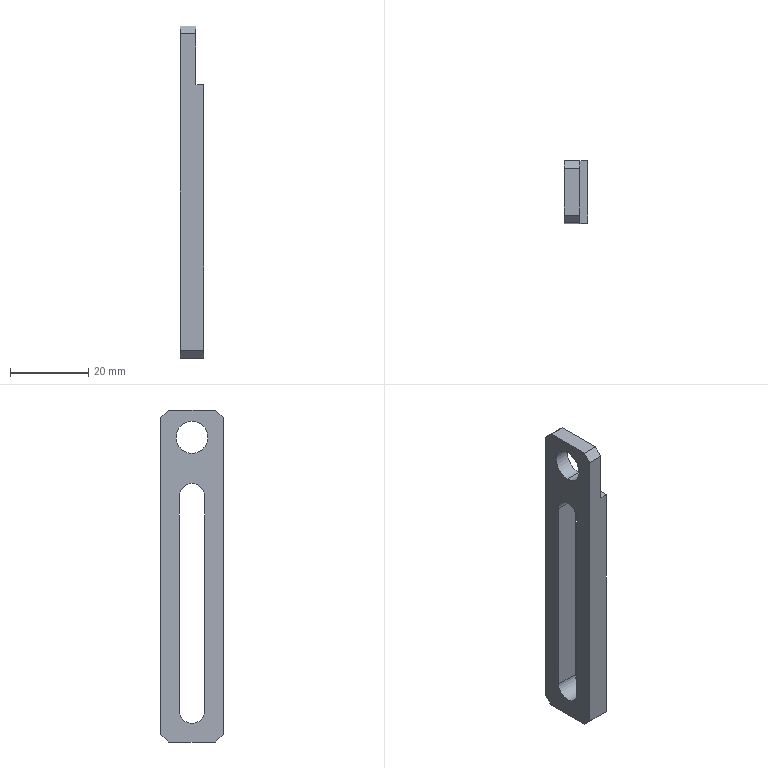Part | SolidWorks | features Chamfer 1, Extrusion 1, HoleWzd 1, ICE 1 | 1 solid | 19 faces | box 6 x 16 x 85 mm | volume 5085 mm3 | plane 14 | cylinder 5 | commonest cylinder face diameters 6.5 x3 8.2 x2
STEP:
#1=CARTESIAN_POINT('',(0.,-8.,-2.9));
#2=VERTEX_POINT('',#1);
#3=CARTESIAN_POINT('',(0.,-8.,-11.1));
#4=VERTEX_POINT('',#3);
#5=CARTESIAN_POINT('',(0.,-8.,-7.));
#6=DIRECTION('',(1.,0.,0.));
#7=DIRECTION('',(0.,0.,-1.));
#8=AXIS2_PLACEMENT_3D('',#5,#6,#7);
#9=CIRCLE('',#8,4.1);
#10=EDGE_CURVE('',#2,#4,#9,.T.);
#11=ORIENTED_EDGE('',*,*,#10,.F.);
#12=CARTESIAN_POINT('',(4.,-8.,-2.9));
#13=VERTEX_POINT('',#12);
#14=CARTESIAN_POINT('',(6.,-8.,-2.9));
#15=DIRECTION('',(1.,0.,0.));
#16=VECTOR('',#15,1000.);
#17=LINE('',#14,#16);
#18=EDGE_CURVE('',#2,#13,#17,.T.);
#19=ORIENTED_EDGE('',*,*,#18,.T.);
#20=CARTESIAN_POINT('',(4.,-8.,-11.1));
#21=VERTEX_POINT('',#20);
#22=CARTESIAN_POINT('',(4.,-8.,-7.));
#23=DIRECTION('',(1.,0.,0.));
#24=DIRECTION('',(0.,0.,1.));
#25=AXIS2_PLACEMENT_3D('',#22,#23,#24);
#26=CIRCLE('',#25,4.1);
#27=EDGE_CURVE('',#13,#21,#26,.T.);
#28=ORIENTED_EDGE('',*,*,#27,.T.);
#29=CARTESIAN_POINT('',(6.,-8.,-11.1));
#30=DIRECTION('',(1.,0.,0.));
#31=VECTOR('',#30,1000.);
#32=LINE('',#29,#31);
#33=EDGE_CURVE('',#4,#21,#32,.T.);
#34=ORIENTED_EDGE('',*,*,#33,.F.);
#35=EDGE_LOOP('',(#11,#19,#28,#34));
#36=FACE_OUTER_BOUND('',#35,.T.);
#37=CARTESIAN_POINT('',(6.,-8.,-7.));
#38=DIRECTION('',(1.,0.,0.));
#39=DIRECTION('',(0.,0.,-1.));
#40=AXIS2_PLACEMENT_3D('',#37,#38,#39);
#41=CYLINDRICAL_SURFACE('',#40,4.1);
#42=ADVANCED_FACE('',(#36),#41,.F.);
#43=CARTESIAN_POINT('',(6.,-4.75,-22.));
#44=VERTEX_POINT('',#43);
#45=CARTESIAN_POINT('',(6.,-8.,-18.75));
#46=VERTEX_POINT('',#45);
#47=CARTESIAN_POINT('',(6.,-8.,-22.));
#48=DIRECTION('',(1.,0.,0.));
#49=DIRECTION('',(0.,0.,-1.));
#50=AXIS2_PLACEMENT_3D('',#47,#48,#49);
#51=CIRCLE('',#50,3.25);
#52=EDGE_CURVE('',#44,#46,#51,.T.);
#53=ORIENTED_EDGE('',*,*,#52,.T.);
#54=CARTESIAN_POINT('',(0.,-8.,-18.75));
#55=VERTEX_POINT('',#54);
#56=CARTESIAN_POINT('',(6.,-8.,-18.75));
#57=DIRECTION('',(-1.,0.,0.));
#58=VECTOR('',#57,1000.);
#59=LINE('',#56,#58);
#60=EDGE_CURVE('',#46,#55,#59,.T.);
#61=ORIENTED_EDGE('',*,*,#60,.T.);
#62=CARTESIAN_POINT('',(0.,-4.75,-22.));
#63=VERTEX_POINT('',#62);
#64=CARTESIAN_POINT('',(0.,-8.,-22.));
#65=DIRECTION('',(1.,0.,0.));
#66=DIRECTION('',(0.,0.,-1.));
#67=AXIS2_PLACEMENT_3D('',#64,#65,#66);
#68=CIRCLE('',#67,3.25);
#69=EDGE_CURVE('',#63,#55,#68,.T.);
#70=ORIENTED_EDGE('',*,*,#69,.F.);
#71=CARTESIAN_POINT('',(6.,-4.75,-22.));
#72=DIRECTION('',(-1.,0.,0.));
#73=VECTOR('',#72,1000.);
#74=LINE('',#71,#73);
#75=EDGE_CURVE('',#44,#63,#74,.T.);
#76=ORIENTED_EDGE('',*,*,#75,.F.);
#77=EDGE_LOOP('',(#53,#61,#70,#76));
#78=FACE_OUTER_BOUND('',#77,.T.);
#79=CARTESIAN_POINT('',(6.,-8.,-22.));
#80=DIRECTION('',(-1.,0.,0.));
#81=DIRECTION('',(0.,0.,1.));
#82=AXIS2_PLACEMENT_3D('',#79,#80,#81);
#83=CYLINDRICAL_SURFACE('',#82,3.25);
#84=ADVANCED_FACE('',(#78),#83,.F.);
#85=CARTESIAN_POINT('',(6.,-16.,-15.));
#86=VERTEX_POINT('',#85);
#87=CARTESIAN_POINT('',(6.,0.,-15.));
#88=VERTEX_POINT('',#87);
#89=CARTESIAN_POINT('',(6.,0.,-15.));
#90=DIRECTION('',(0.,1.,0.));
#91=VECTOR('',#90,1000.);
#92=LINE('',#89,#91);
#93=EDGE_CURVE('',#86,#88,#92,.T.);
#94=ORIENTED_EDGE('',*,*,#93,.F.);
#95=CARTESIAN_POINT('',(6.,-16.,-83.));
#96=VERTEX_POINT('',#95);
#97=CARTESIAN_POINT('',(6.,-16.,0.));
#98=DIRECTION('',(0.,0.,-1.));
#99=VECTOR('',#98,1000.);
#100=LINE('',#97,#99);
#101=EDGE_CURVE('',#86,#96,#100,.T.);
#102=ORIENTED_EDGE('',*,*,#101,.T.);
#103=CARTESIAN_POINT('',(6.,-14.,-85.));
#104=VERTEX_POINT('',#103);
#105=CARTESIAN_POINT('',(6.,-57.5,-41.5));
#106=DIRECTION('',(0.,0.7071,-0.7071));
#107=VECTOR('',#106,1000.);
#108=LINE('',#105,#107);
#109=EDGE_CURVE('',#96,#104,#108,.T.);
#110=ORIENTED_EDGE('',*,*,#109,.T.);
#111=CARTESIAN_POINT('',(6.,-2.,-85.));
#112=VERTEX_POINT('',#111);
#113=CARTESIAN_POINT('',(6.,0.,-85.));
#114=DIRECTION('',(0.,1.,0.));
#115=VECTOR('',#114,1000.);
#116=LINE('',#113,#115);
#117=EDGE_CURVE('',#104,#112,#116,.T.);
#118=ORIENTED_EDGE('',*,*,#117,.T.);
#119=CARTESIAN_POINT('',(6.,0.,-83.));
#120=VERTEX_POINT('',#119);
#121=CARTESIAN_POINT('',(6.,33.5,-49.5));
#122=DIRECTION('',(0.,0.7071,0.7071));
#123=VECTOR('',#122,1000.);
#124=LINE('',#121,#123);
#125=EDGE_CURVE('',#112,#120,#124,.T.);
#126=ORIENTED_EDGE('',*,*,#125,.T.);
#127=CARTESIAN_POINT('',(6.,0.,0.));
#128=DIRECTION('',(0.,0.,1.));
#129=VECTOR('',#128,1000.);
#130=LINE('',#127,#129);
#131=EDGE_CURVE('',#120,#88,#130,.T.);
#132=ORIENTED_EDGE('',*,*,#131,.T.);
#133=EDGE_LOOP('',(#94,#102,#110,#118,#126,#132));
#134=FACE_OUTER_BOUND('',#133,.T.);
#135=CARTESIAN_POINT('',(6.,-11.25,-22.));
#136=VERTEX_POINT('',#135);
#137=CARTESIAN_POINT('',(6.,-11.25,-77.));
#138=VERTEX_POINT('',#137);
#139=CARTESIAN_POINT('',(6.,-11.25,-22.));
#140=DIRECTION('',(0.,0.,-1.));
#141=VECTOR('',#140,1000.);
#142=LINE('',#139,#141);
#143=EDGE_CURVE('',#136,#138,#142,.T.);
#144=ORIENTED_EDGE('',*,*,#143,.F.);
#145=CARTESIAN_POINT('',(6.,-8.,-22.));
#146=DIRECTION('',(1.,0.,0.));
#147=DIRECTION('',(0.,0.,-1.));
#148=AXIS2_PLACEMENT_3D('',#145,#146,#147);
#149=CIRCLE('',#148,3.25);
#150=EDGE_CURVE('',#46,#136,#149,.T.);
#151=ORIENTED_EDGE('',*,*,#150,.F.);
#152=ORIENTED_EDGE('',*,*,#52,.F.);
#153=CARTESIAN_POINT('',(6.,-4.75,-77.));
#154=VERTEX_POINT('',#153);
#155=CARTESIAN_POINT('',(6.,-4.75,-22.));
#156=DIRECTION('',(0.,0.,1.));
#157=VECTOR('',#156,1000.);
#158=LINE('',#155,#157);
#159=EDGE_CURVE('',#154,#44,#158,.T.);
#160=ORIENTED_EDGE('',*,*,#159,.F.);
#161=CARTESIAN_POINT('',(6.,-8.,-77.));
#162=DIRECTION('',(1.,0.,0.));
#163=DIRECTION('',(0.,0.,-1.));
#164=AXIS2_PLACEMENT_3D('',#161,#162,#163);
#165=CIRCLE('',#164,3.25);
#166=EDGE_CURVE('',#138,#154,#165,.T.);
#167=ORIENTED_EDGE('',*,*,#166,.F.);
#168=EDGE_LOOP('',(#144,#151,#152,#160,#167));
#169=FACE_BOUND('',#168,.T.);
#170=CARTESIAN_POINT('',(6.,-16.,0.));
#171=DIRECTION('',(1.,0.,0.));
#172=DIRECTION('',(0.,0.,-1.));
#173=AXIS2_PLACEMENT_3D('',#170,#171,#172);
#174=PLANE('',#173);
#175=ADVANCED_FACE('',(#134,#169),#174,.T.);
#176=CARTESIAN_POINT('',(0.,-8.,-7.));
#177=DIRECTION('',(1.,0.,0.));
#178=DIRECTION('',(0.,0.,-1.));
#179=AXIS2_PLACEMENT_3D('',#176,#177,#178);
#180=CIRCLE('',#179,4.1);
#181=EDGE_CURVE('',#4,#2,#180,.T.);
#182=ORIENTED_EDGE('',*,*,#181,.T.);
#183=ORIENTED_EDGE('',*,*,#10,.T.);
#184=EDGE_LOOP('',(#182,#183));
#185=FACE_BOUND('',#184,.T.);
#186=CARTESIAN_POINT('',(0.,0.,-83.));
#187=VERTEX_POINT('',#186);
#188=CARTESIAN_POINT('',(0.,0.,-2.));
#189=VERTEX_POINT('',#188);
#190=CARTESIAN_POINT('',(0.,0.,0.));
#191=DIRECTION('',(0.,0.,1.));
#192=VECTOR('',#191,1000.);
#193=LINE('',#190,#192);
#194=EDGE_CURVE('',#187,#189,#193,.T.);
#195=ORIENTED_EDGE('',*,*,#194,.F.);
#196=CARTESIAN_POINT('',(0.,-2.,-85.));
#197=VERTEX_POINT('',#196);
#198=CARTESIAN_POINT('',(0.,0.,-83.));
#199=DIRECTION('',(0.,-0.7071,-0.7071));
#200=VECTOR('',#199,1000.);
#201=LINE('',#198,#200);
#202=EDGE_CURVE('',#187,#197,#201,.T.);
#203=ORIENTED_EDGE('',*,*,#202,.T.);
#204=CARTESIAN_POINT('',(0.,-14.,-85.));
#205=VERTEX_POINT('',#204);
#206=CARTESIAN_POINT('',(0.,0.,-85.));
#207=DIRECTION('',(0.,1.,0.));
#208=VECTOR('',#207,1000.);
#209=LINE('',#206,#208);
#210=EDGE_CURVE('',#205,#197,#209,.T.);
#211=ORIENTED_EDGE('',*,*,#210,.F.);
#212=CARTESIAN_POINT('',(0.,-16.,-83.));
#213=VERTEX_POINT('',#212);
#214=CARTESIAN_POINT('',(0.,-14.,-85.));
#215=DIRECTION('',(0.,-0.7071,0.7071));
#216=VECTOR('',#215,1000.);
#217=LINE('',#214,#216);
#218=EDGE_CURVE('',#205,#213,#217,.T.);
#219=ORIENTED_EDGE('',*,*,#218,.T.);
#220=CARTESIAN_POINT('',(0.,-16.,-2.));
#221=VERTEX_POINT('',#220);
#222=CARTESIAN_POINT('',(0.,-16.,0.));
#223=DIRECTION('',(0.,0.,-1.));
#224=VECTOR('',#223,1000.);
#225=LINE('',#222,#224);
#226=EDGE_CURVE('',#221,#213,#225,.T.);
#227=ORIENTED_EDGE('',*,*,#226,.F.);
#228=CARTESIAN_POINT('',(0.,-14.,0.));
#229=VERTEX_POINT('',#228);
#230=CARTESIAN_POINT('',(0.,-16.,-2.));
#231=DIRECTION('',(0.,0.7071,0.7071));
#232=VECTOR('',#231,1000.);
#233=LINE('',#230,#232);
#234=EDGE_CURVE('',#221,#229,#233,.T.);
#235=ORIENTED_EDGE('',*,*,#234,.T.);
#236=CARTESIAN_POINT('',(0.,-2.,0.));
#237=VERTEX_POINT('',#236);
#238=CARTESIAN_POINT('',(0.,0.,0.));
#239=DIRECTION('',(0.,-1.,0.));
#240=VECTOR('',#239,1000.);
#241=LINE('',#238,#240);
#242=EDGE_CURVE('',#237,#229,#241,.T.);
#243=ORIENTED_EDGE('',*,*,#242,.F.);
#244=CARTESIAN_POINT('',(0.,-2.,0.));
#245=DIRECTION('',(0.,0.7071,-0.7071));
#246=VECTOR('',#245,1000.);
#247=LINE('',#244,#246);
#248=EDGE_CURVE('',#237,#189,#247,.T.);
#249=ORIENTED_EDGE('',*,*,#248,.T.);
#250=EDGE_LOOP('',(#195,#203,#211,#219,#227,#235,#243,#249));
#251=FACE_OUTER_BOUND('',#250,.T.);
#252=ORIENTED_EDGE('',*,*,#69,.T.);
#253=CARTESIAN_POINT('',(0.,-11.25,-22.));
#254=VERTEX_POINT('',#253);
#255=CARTESIAN_POINT('',(0.,-8.,-22.));
#256=DIRECTION('',(1.,0.,0.));
#257=DIRECTION('',(0.,0.,-1.));
#258=AXIS2_PLACEMENT_3D('',#255,#256,#257);
#259=CIRCLE('',#258,3.25);
#260=EDGE_CURVE('',#55,#254,#259,.T.);
#261=ORIENTED_EDGE('',*,*,#260,.T.);
#262=CARTESIAN_POINT('',(0.,-11.25,-77.));
#263=VERTEX_POINT('',#262);
#264=CARTESIAN_POINT('',(0.,-11.25,-22.));
#265=DIRECTION('',(0.,0.,-1.));
#266=VECTOR('',#265,1000.);
#267=LINE('',#264,#266);
#268=EDGE_CURVE('',#254,#263,#267,.T.);
#269=ORIENTED_EDGE('',*,*,#268,.T.);
#270=CARTESIAN_POINT('',(0.,-4.75,-77.));
#271=VERTEX_POINT('',#270);
#272=CARTESIAN_POINT('',(0.,-8.,-77.));
#273=DIRECTION('',(1.,0.,0.));
#274=DIRECTION('',(0.,0.,-1.));
#275=AXIS2_PLACEMENT_3D('',#272,#273,#274);
#276=CIRCLE('',#275,3.25);
#277=EDGE_CURVE('',#263,#271,#276,.T.);
#278=ORIENTED_EDGE('',*,*,#277,.T.);
#279=CARTESIAN_POINT('',(0.,-4.75,-22.));
#280=DIRECTION('',(0.,0.,1.));
#281=VECTOR('',#280,1000.);
#282=LINE('',#279,#281);
#283=EDGE_CURVE('',#271,#63,#282,.T.);
#284=ORIENTED_EDGE('',*,*,#283,.T.);
#285=EDGE_LOOP('',(#252,#261,#269,#278,#284));
#286=FACE_BOUND('',#285,.T.);
#287=CARTESIAN_POINT('',(0.,-16.,0.));
#288=DIRECTION('',(1.,0.,0.));
#289=DIRECTION('',(0.,0.,-1.));
#290=AXIS2_PLACEMENT_3D('',#287,#288,#289);
#291=PLANE('',#290);
#292=ADVANCED_FACE('',(#185,#251,#286),#291,.F.);
#293=CARTESIAN_POINT('',(4.,-14.,0.));
#294=VERTEX_POINT('',#293);
#295=CARTESIAN_POINT('',(6.,-14.,0.));
#296=DIRECTION('',(1.,0.,0.));
#297=VECTOR('',#296,1000.);
#298=LINE('',#295,#297);
#299=EDGE_CURVE('',#229,#294,#298,.T.);
#300=ORIENTED_EDGE('',*,*,#299,.T.);
#301=CARTESIAN_POINT('',(4.,-2.,0.));
#302=VERTEX_POINT('',#301);
#303=CARTESIAN_POINT('',(4.,0.,0.));
#304=DIRECTION('',(0.,-1.,0.));
#305=VECTOR('',#304,1000.);
#306=LINE('',#303,#305);
#307=EDGE_CURVE('',#302,#294,#306,.T.);
#308=ORIENTED_EDGE('',*,*,#307,.F.);
#309=CARTESIAN_POINT('',(6.,-2.,0.));
#310=DIRECTION('',(-1.,0.,0.));
#311=VECTOR('',#310,1000.);
#312=LINE('',#309,#311);
#313=EDGE_CURVE('',#302,#237,#312,.T.);
#314=ORIENTED_EDGE('',*,*,#313,.T.);
#315=ORIENTED_EDGE('',*,*,#242,.T.);
#316=EDGE_LOOP('',(#300,#308,#314,#315));
#317=FACE_OUTER_BOUND('',#316,.T.);
#318=CARTESIAN_POINT('',(6.,0.,0.));
#319=DIRECTION('',(0.,0.,-1.));
#320=DIRECTION('',(0.,1.,0.));
#321=AXIS2_PLACEMENT_3D('',#318,#319,#320);
#322=PLANE('',#321);
#323=ADVANCED_FACE('',(#317),#322,.F.);
#324=ORIENTED_EDGE('',*,*,#101,.F.);
#325=CARTESIAN_POINT('',(4.,-16.,-15.));
#326=VERTEX_POINT('',#325);
#327=CARTESIAN_POINT('',(4.,-16.,-15.));
#328=DIRECTION('',(1.,0.,0.));
#329=VECTOR('',#328,1000.);
#330=LINE('',#327,#329);
#331=EDGE_CURVE('',#326,#86,#330,.T.);
#332=ORIENTED_EDGE('',*,*,#331,.F.);
#333=CARTESIAN_POINT('',(4.,-16.,-2.));
#334=VERTEX_POINT('',#333);
#335=CARTESIAN_POINT('',(4.,-16.,-15.));
#336=DIRECTION('',(0.,0.,-1.));
#337=VECTOR('',#336,1000.);
#338=LINE('',#335,#337);
#339=EDGE_CURVE('',#334,#326,#338,.T.);
#340=ORIENTED_EDGE('',*,*,#339,.F.);
#341=CARTESIAN_POINT('',(6.,-16.,-2.));
#342=DIRECTION('',(-1.,0.,0.));
#343=VECTOR('',#342,1000.);
#344=LINE('',#341,#343);
#345=EDGE_CURVE('',#334,#221,#344,.T.);
#346=ORIENTED_EDGE('',*,*,#345,.T.);
#347=ORIENTED_EDGE('',*,*,#226,.T.);
#348=CARTESIAN_POINT('',(6.,-16.,-83.));
#349=DIRECTION('',(1.,0.,0.));
#350=VECTOR('',#349,1000.);
#351=LINE('',#348,#350);
#352=EDGE_CURVE('',#213,#96,#351,.T.);
#353=ORIENTED_EDGE('',*,*,#352,.T.);
#354=EDGE_LOOP('',(#324,#332,#340,#346,#347,#353));
#355=FACE_OUTER_BOUND('',#354,.T.);
#356=CARTESIAN_POINT('',(6.,-16.,0.));
#357=DIRECTION('',(0.,1.,0.));
#358=DIRECTION('',(0.,0.,1.));
#359=AXIS2_PLACEMENT_3D('',#356,#357,#358);
#360=PLANE('',#359);
#361=ADVANCED_FACE('',(#355),#360,.F.);
#362=ORIENTED_EDGE('',*,*,#210,.T.);
#363=CARTESIAN_POINT('',(6.,-2.,-85.));
#364=DIRECTION('',(1.,0.,0.));
#365=VECTOR('',#364,1000.);
#366=LINE('',#363,#365);
#367=EDGE_CURVE('',#197,#112,#366,.T.);
#368=ORIENTED_EDGE('',*,*,#367,.T.);
#369=ORIENTED_EDGE('',*,*,#117,.F.);
#370=CARTESIAN_POINT('',(6.,-14.,-85.));
#371=DIRECTION('',(-1.,0.,0.));
#372=VECTOR('',#371,1000.);
#373=LINE('',#370,#372);
#374=EDGE_CURVE('',#104,#205,#373,.T.);
#375=ORIENTED_EDGE('',*,*,#374,.T.);
#376=EDGE_LOOP('',(#362,#368,#369,#375));
#377=FACE_OUTER_BOUND('',#376,.T.);
#378=CARTESIAN_POINT('',(6.,0.,-85.));
#379=DIRECTION('',(0.,0.,1.));
#380=DIRECTION('',(1.,0.,0.));
#381=AXIS2_PLACEMENT_3D('',#378,#379,#380);
#382=PLANE('',#381);
#383=ADVANCED_FACE('',(#377),#382,.F.);
#384=CARTESIAN_POINT('',(4.,0.,-15.));
#385=VERTEX_POINT('',#384);
#386=CARTESIAN_POINT('',(4.,0.,-2.));
#387=VERTEX_POINT('',#386);
#388=CARTESIAN_POINT('',(4.,0.,-15.));
#389=DIRECTION('',(0.,0.,1.));
#390=VECTOR('',#389,1000.);
#391=LINE('',#388,#390);
#392=EDGE_CURVE('',#385,#387,#391,.T.);
#393=ORIENTED_EDGE('',*,*,#392,.F.);
#394=CARTESIAN_POINT('',(4.,0.,-15.));
#395=DIRECTION('',(1.,0.,0.));
#396=VECTOR('',#395,1000.);
#397=LINE('',#394,#396);
#398=EDGE_CURVE('',#385,#88,#397,.T.);
#399=ORIENTED_EDGE('',*,*,#398,.T.);
#400=ORIENTED_EDGE('',*,*,#131,.F.);
#401=CARTESIAN_POINT('',(6.,0.,-83.));
#402=DIRECTION('',(-1.,0.,0.));
#403=VECTOR('',#402,1000.);
#404=LINE('',#401,#403);
#405=EDGE_CURVE('',#120,#187,#404,.T.);
#406=ORIENTED_EDGE('',*,*,#405,.T.);
#407=ORIENTED_EDGE('',*,*,#194,.T.);
#408=CARTESIAN_POINT('',(6.,0.,-2.));
#409=DIRECTION('',(1.,0.,0.));
#410=VECTOR('',#409,1000.);
#411=LINE('',#408,#410);
#412=EDGE_CURVE('',#189,#387,#411,.T.);
#413=ORIENTED_EDGE('',*,*,#412,.T.);
#414=EDGE_LOOP('',(#393,#399,#400,#406,#407,#413));
#415=FACE_OUTER_BOUND('',#414,.T.);
#416=CARTESIAN_POINT('',(6.,0.,0.));
#417=DIRECTION('',(0.,-1.,0.));
#418=DIRECTION('',(0.,0.,-1.));
#419=AXIS2_PLACEMENT_3D('',#416,#417,#418);
#420=PLANE('',#419);
#421=ADVANCED_FACE('',(#415),#420,.F.);
#422=ORIENTED_EDGE('',*,*,#60,.F.);
#423=ORIENTED_EDGE('',*,*,#150,.T.);
#424=CARTESIAN_POINT('',(6.,-11.25,-22.));
#425=DIRECTION('',(-1.,0.,0.));
#426=VECTOR('',#425,1000.);
#427=LINE('',#424,#426);
#428=EDGE_CURVE('',#136,#254,#427,.T.);
#429=ORIENTED_EDGE('',*,*,#428,.T.);
#430=ORIENTED_EDGE('',*,*,#260,.F.);
#431=EDGE_LOOP('',(#422,#423,#429,#430));
#432=FACE_OUTER_BOUND('',#431,.T.);
#433=CARTESIAN_POINT('',(6.,-8.,-22.));
#434=DIRECTION('',(-1.,0.,0.));
#435=DIRECTION('',(0.,0.,1.));
#436=AXIS2_PLACEMENT_3D('',#433,#434,#435);
#437=CYLINDRICAL_SURFACE('',#436,3.25);
#438=ADVANCED_FACE('',(#432),#437,.F.);
#439=ORIENTED_EDGE('',*,*,#268,.F.);
#440=ORIENTED_EDGE('',*,*,#428,.F.);
#441=ORIENTED_EDGE('',*,*,#143,.T.);
#442=CARTESIAN_POINT('',(6.,-11.25,-77.));
#443=DIRECTION('',(-1.,0.,0.));
#444=VECTOR('',#443,1000.);
#445=LINE('',#442,#444);
#446=EDGE_CURVE('',#138,#263,#445,.T.);
#447=ORIENTED_EDGE('',*,*,#446,.T.);
#448=EDGE_LOOP('',(#439,#440,#441,#447));
#449=FACE_OUTER_BOUND('',#448,.T.);
#450=CARTESIAN_POINT('',(6.,-11.25,-22.));
#451=DIRECTION('',(0.,1.,0.));
#452=DIRECTION('',(0.,0.,1.));
#453=AXIS2_PLACEMENT_3D('',#450,#451,#452);
#454=PLANE('',#453);
#455=ADVANCED_FACE('',(#449),#454,.T.);
#456=ORIENTED_EDGE('',*,*,#277,.F.);
#457=ORIENTED_EDGE('',*,*,#446,.F.);
#458=ORIENTED_EDGE('',*,*,#166,.T.);
#459=CARTESIAN_POINT('',(6.,-4.75,-77.));
#460=DIRECTION('',(-1.,0.,0.));
#461=VECTOR('',#460,1000.);
#462=LINE('',#459,#461);
#463=EDGE_CURVE('',#154,#271,#462,.T.);
#464=ORIENTED_EDGE('',*,*,#463,.T.);
#465=EDGE_LOOP('',(#456,#457,#458,#464));
#466=FACE_OUTER_BOUND('',#465,.T.);
#467=CARTESIAN_POINT('',(6.,-8.,-77.));
#468=DIRECTION('',(-1.,0.,0.));
#469=DIRECTION('',(0.,0.,1.));
#470=AXIS2_PLACEMENT_3D('',#467,#468,#469);
#471=CYLINDRICAL_SURFACE('',#470,3.25);
#472=ADVANCED_FACE('',(#466),#471,.F.);
#473=ORIENTED_EDGE('',*,*,#283,.F.);
#474=ORIENTED_EDGE('',*,*,#463,.F.);
#475=ORIENTED_EDGE('',*,*,#159,.T.);
#476=ORIENTED_EDGE('',*,*,#75,.T.);
#477=EDGE_LOOP('',(#473,#474,#475,#476));
#478=FACE_OUTER_BOUND('',#477,.T.);
#479=CARTESIAN_POINT('',(6.,-4.75,-22.));
#480=DIRECTION('',(0.,-1.,0.));
#481=DIRECTION('',(0.,0.,-1.));
#482=AXIS2_PLACEMENT_3D('',#479,#480,#481);
#483=PLANE('',#482);
#484=ADVANCED_FACE('',(#478),#483,.T.);
#485=ORIENTED_EDGE('',*,*,#18,.F.);
#486=ORIENTED_EDGE('',*,*,#181,.F.);
#487=ORIENTED_EDGE('',*,*,#33,.T.);
#488=CARTESIAN_POINT('',(4.,-8.,-7.));
#489=DIRECTION('',(1.,0.,0.));
#490=DIRECTION('',(0.,0.,1.));
#491=AXIS2_PLACEMENT_3D('',#488,#489,#490);
#492=CIRCLE('',#491,4.1);
#493=EDGE_CURVE('',#21,#13,#492,.T.);
#494=ORIENTED_EDGE('',*,*,#493,.T.);
#495=EDGE_LOOP('',(#485,#486,#487,#494));
#496=FACE_OUTER_BOUND('',#495,.T.);
#497=CARTESIAN_POINT('',(6.,-8.,-7.));
#498=DIRECTION('',(1.,0.,0.));
#499=DIRECTION('',(0.,0.,-1.));
#500=AXIS2_PLACEMENT_3D('',#497,#498,#499);
#501=CYLINDRICAL_SURFACE('',#500,4.1);
#502=ADVANCED_FACE('',(#496),#501,.F.);
#503=ORIENTED_EDGE('',*,*,#125,.F.);
#504=ORIENTED_EDGE('',*,*,#367,.F.);
#505=ORIENTED_EDGE('',*,*,#202,.F.);
#506=ORIENTED_EDGE('',*,*,#405,.F.);
#507=EDGE_LOOP('',(#503,#504,#505,#506));
#508=FACE_OUTER_BOUND('',#507,.T.);
#509=CARTESIAN_POINT('',(6.,0.,-83.));
#510=DIRECTION('',(0.,-0.7071,0.7071));
#511=DIRECTION('',(0.,-0.7071,-0.7071));
#512=AXIS2_PLACEMENT_3D('',#509,#510,#511);
#513=PLANE('',#512);
#514=ADVANCED_FACE('',(#508),#513,.F.);
#515=ORIENTED_EDGE('',*,*,#109,.F.);
#516=ORIENTED_EDGE('',*,*,#352,.F.);
#517=ORIENTED_EDGE('',*,*,#218,.F.);
#518=ORIENTED_EDGE('',*,*,#374,.F.);
#519=EDGE_LOOP('',(#515,#516,#517,#518));
#520=FACE_OUTER_BOUND('',#519,.T.);
#521=CARTESIAN_POINT('',(6.,-14.,-85.));
#522=DIRECTION('',(0.,0.7071,0.7071));
#523=DIRECTION('',(0.,-0.7071,0.7071));
#524=AXIS2_PLACEMENT_3D('',#521,#522,#523);
#525=PLANE('',#524);
#526=ADVANCED_FACE('',(#520),#525,.F.);
#527=CARTESIAN_POINT('',(4.,-16.,-2.));
#528=DIRECTION('',(0.,-0.7071,-0.7071));
#529=VECTOR('',#528,1000.);
#530=LINE('',#527,#529);
#531=EDGE_CURVE('',#294,#334,#530,.T.);
#532=ORIENTED_EDGE('',*,*,#531,.F.);
#533=ORIENTED_EDGE('',*,*,#299,.F.);
#534=ORIENTED_EDGE('',*,*,#234,.F.);
#535=ORIENTED_EDGE('',*,*,#345,.F.);
#536=EDGE_LOOP('',(#532,#533,#534,#535));
#537=FACE_OUTER_BOUND('',#536,.T.);
#538=CARTESIAN_POINT('',(6.,-16.,-2.));
#539=DIRECTION('',(0.,0.7071,-0.7071));
#540=DIRECTION('',(0.,0.7071,0.7071));
#541=AXIS2_PLACEMENT_3D('',#538,#539,#540);
#542=PLANE('',#541);
#543=ADVANCED_FACE('',(#537),#542,.F.);
#544=CARTESIAN_POINT('',(4.,-2.,0.));
#545=DIRECTION('',(0.,-0.7071,0.7071));
#546=VECTOR('',#545,1000.);
#547=LINE('',#544,#546);
#548=EDGE_CURVE('',#387,#302,#547,.T.);
#549=ORIENTED_EDGE('',*,*,#548,.F.);
#550=ORIENTED_EDGE('',*,*,#412,.F.);
#551=ORIENTED_EDGE('',*,*,#248,.F.);
#552=ORIENTED_EDGE('',*,*,#313,.F.);
#553=EDGE_LOOP('',(#549,#550,#551,#552));
#554=FACE_OUTER_BOUND('',#553,.T.);
#555=CARTESIAN_POINT('',(6.,-2.,0.));
#556=DIRECTION('',(0.,-0.7071,-0.7071));
#557=DIRECTION('',(0.,0.7071,-0.7071));
#558=AXIS2_PLACEMENT_3D('',#555,#556,#557);
#559=PLANE('',#558);
#560=ADVANCED_FACE('',(#554),#559,.F.);
#561=ORIENTED_EDGE('',*,*,#531,.T.);
#562=ORIENTED_EDGE('',*,*,#339,.T.);
#563=CARTESIAN_POINT('',(4.,0.,-15.));
#564=DIRECTION('',(0.,1.,0.));
#565=VECTOR('',#564,1000.);
#566=LINE('',#563,#565);
#567=EDGE_CURVE('',#326,#385,#566,.T.);
#568=ORIENTED_EDGE('',*,*,#567,.T.);
#569=ORIENTED_EDGE('',*,*,#392,.T.);
#570=ORIENTED_EDGE('',*,*,#548,.T.);
#571=ORIENTED_EDGE('',*,*,#307,.T.);
#572=EDGE_LOOP('',(#561,#562,#568,#569,#570,#571));
#573=FACE_OUTER_BOUND('',#572,.T.);
#574=ORIENTED_EDGE('',*,*,#493,.F.);
#575=ORIENTED_EDGE('',*,*,#27,.F.);
#576=EDGE_LOOP('',(#574,#575));
#577=FACE_BOUND('',#576,.T.);
#578=CARTESIAN_POINT('',(4.,0.,0.));
#579=DIRECTION('',(-1.,0.,0.));
#580=DIRECTION('',(0.,0.,1.));
#581=AXIS2_PLACEMENT_3D('',#578,#579,#580);
#582=PLANE('',#581);
#583=ADVANCED_FACE('',(#573,#577),#582,.F.);
#584=ORIENTED_EDGE('',*,*,#93,.T.);
#585=ORIENTED_EDGE('',*,*,#398,.F.);
#586=ORIENTED_EDGE('',*,*,#567,.F.);
#587=ORIENTED_EDGE('',*,*,#331,.T.);
#588=EDGE_LOOP('',(#584,#585,#586,#587));
#589=FACE_OUTER_BOUND('',#588,.T.);
#590=CARTESIAN_POINT('',(4.,0.,-15.));
#591=DIRECTION('',(0.,0.,-1.));
#592=DIRECTION('',(0.,1.,0.));
#593=AXIS2_PLACEMENT_3D('',#590,#591,#592);
#594=PLANE('',#593);
#595=ADVANCED_FACE('',(#589),#594,.F.);
#596=CLOSED_SHELL('',(#42,#84,#175,#292,#323,#361,#383,#421,#438,#455,#472,#484,#502,#514,#526,#543,#560,#583,#595));
#597=MANIFOLD_SOLID_BREP('',#596);
#598=CARTESIAN_POINT('',(0.,0.,0.));
#599=DIRECTION('',(0.,0.,1.));
#600=DIRECTION('',(1.,0.,0.));
#601=AXIS2_PLACEMENT_3D('',#598,#599,#600);
#602=(LENGTH_UNIT()NAMED_UNIT(*)SI_UNIT(.MILLI.,.METRE.));
#603=UNCERTAINTY_MEASURE_WITH_UNIT(LENGTH_MEASURE(0.00001),#602,'','');
#604=(NAMED_UNIT(*)PLANE_ANGLE_UNIT()SI_UNIT($,.RADIAN.));
#605=(NAMED_UNIT(*)SI_UNIT($,.STERADIAN.)SOLID_ANGLE_UNIT());
#606=(GEOMETRIC_REPRESENTATION_CONTEXT(3)GLOBAL_UNCERTAINTY_ASSIGNED_CONTEXT((#603))GLOBAL_UNIT_ASSIGNED_CONTEXT((#602,#604,#605))REPRESENTATION_CONTEXT('',''));
#607=ADVANCED_BREP_SHAPE_REPRESENTATION('',(#597,#601),#606);